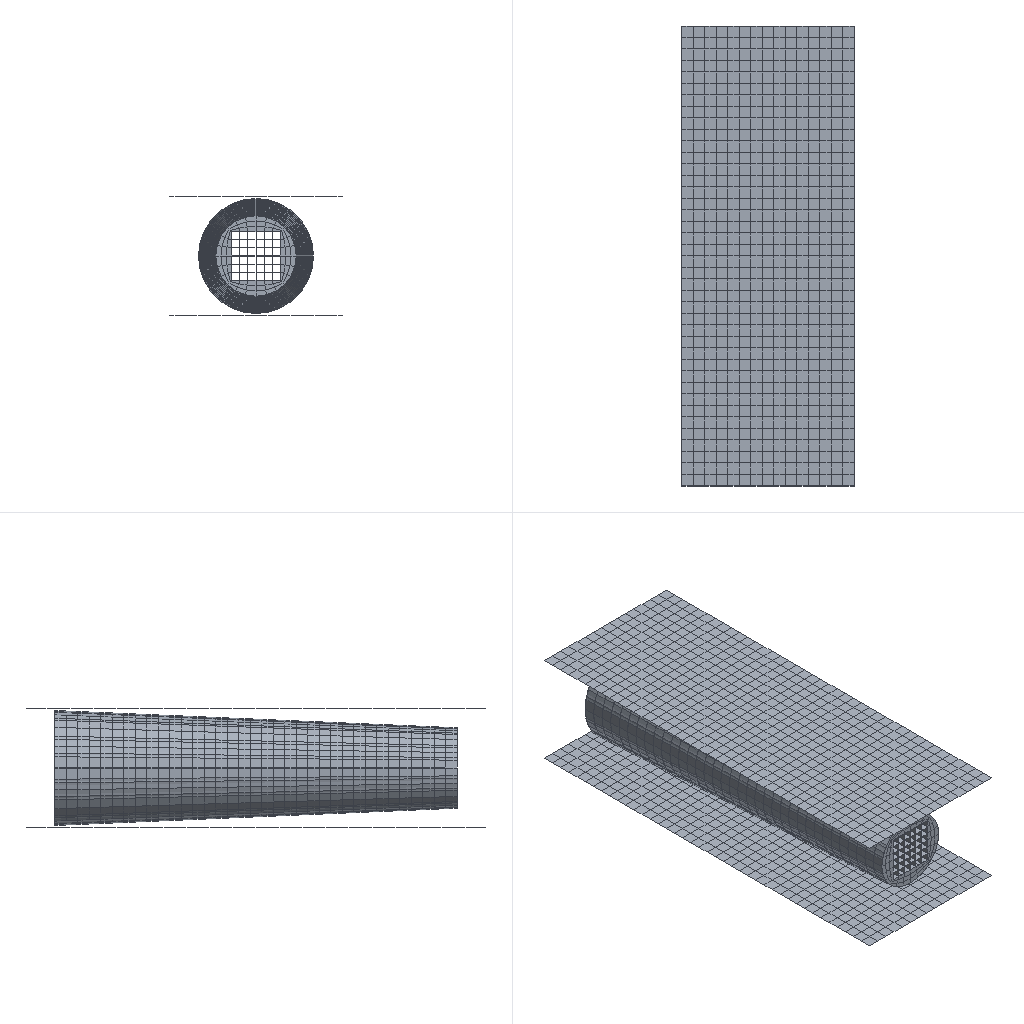Simulation study | abaqus
Set-up summary:
category,name,step,type,value,unit,region
solver,abaqus
solver,version,,,Abaqus/Explicit 2020
units,not stated in the deck,,not stated
analysis,deck,,transient,transient
load_step,Step-1,Step-1,transient
load_step,requested,,,1
mesh,nodes,,,8118
mesh,elements,,,7501
element_type,S4R,,shell,4980
element_type,MASS,,point,1
element_type,C3D8R,,solid,2520
load,load commands in deck,,count,1
bc,support commands in deck,,count,1
material,LV,,in results
material,PU,,in results
material,RIG,,in results
check,setup vs results,,match,"per instance, exact: element labels, types and connectivity; labels of the nodes the elements use; coordinates of those nodes at SINGLE_PRECISION in 4 of 6 instance(s)"
Abaqus input file, long lists of numbers shortened:
*Heading
** Job name: Job-1 Model name: Model-1
** Generated by: Abaqus/CAE 2020
*Preprint, echo=NO, model=NO, history=NO, contact=NO
**
** PARTS
**
*Part, name=ZFX
*Node
      1,         -14.,         -14.,         350.
      2,         -14.,         -14.,           0.
** (1618 more lines like these left out)
*Element, type=S4R
 1,   1,  91, 158,   4
 2,  91,  92, 157, 158
** (2098 more lines like these left out)
*Nset, nset=Set-1
    1,    2,    5,    6,    7,    8,    9,   10,   11,   12,   17,   18,   29,   30,   31,   32
   33,   34,   35,   36,   37,   38,   39,   40,   41,   42,   43,   44,   45,   46,   49,   50
** (75 more lines like these left out)
*Elset, elset=Set-1
   36,   37,   38,   39,   40,   41,   42,   43,   44,   45,   46,   47,   48,   49,   50,   51
   52,   53,   54,   55,   56,   57,   58,   59,   60,   61,   62,   63,   64,   65,   66,   67
** (71 more lines like these left out)
*Nset, nset=Set-2, generate
    1,  1620,     1
*Elset, elset=Set-2, generate
    1,  2100,     1
** Section: zfx
*Shell Section, elset=Set-2, material=LV
0.5, 5
*End Part
**
*Part, name=chongjimian
*Node
      1,        -200.,         -75.,           0.
      2,        -190.,         -75.,           0.
** (654 more lines like these left out)
*Element, type=S4R
  1,   1,   2,  43,  42
  2,   2,   3,  44,  43
** (598 more lines like these left out)
*Node
    657,           0.,           0.,           0.
*Nset, nset=chongjimian-RefPt_, internal
657,
*Nset, nset=Set-1
 657,
*Nset, nset=Set-4, generate
   1,  656,    1
*Elset, elset=Set-4, generate
   1,  600,    1
** Section: rig
*Shell Section, elset=Set-4, material=rig
1., 5
*Element, type=MASS, elset=Set-1_Inertia-1_
601, 657
*Mass, elset=Set-1_Inertia-1_
0.5,
*End Part
**
*Part, name=dimian
*Node
      1,        -200.,         -75.,           0.
      2,        -190.,         -75.,           0.
** (654 more lines like these left out)
*Element, type=S4R
  1,   1,   2,  43,  42
  2,   2,   3,  44,  43
** (598 more lines like these left out)
*Node
    657,           0.,           0.,           0.
*Nset, nset=dimian-RefPt_, internal
657,
*Nset, nset=Set-2, generate
   1,  656,    1
*Elset, elset=Set-2, generate
   1,  600,    1
** Section: rig
*Shell Section, elset=Set-2, material=rig
1., 5
*End Part
**
*Part, name=dpm2
*Node
      1,         -21.,           0.,         -21.
      2,          21.,           0.,         -21.
** (3454 more lines like these left out)
*Element, type=C3D8R
  1,  180,  895, 2097,  759,    1,   23,  419,  100
  2,  895,  896, 2098, 2097,   23,   24,  420,  419
** (2518 more lines like these left out)
*Nset, nset=Set-1, generate
    1,  3456,     1
*Elset, elset=Set-1, generate
    1,  2520,     1
** Section: PU
*Solid Section, elset=Set-1, material=PU
,
*End Part
**
*Part, name=fangguan
*Node
      1,         -21.,         -21.,         350.
      2,         -21.,          21.,         350.
** (574 more lines like these left out)
*Element, type=S4R
  1,   1,   9, 169,  82
  2,   9,  10, 170, 169
** (558 more lines like these left out)
*Nset, nset=Set-1, generate
   1,  576,    1
*Elset, elset=Set-1, generate
   1,  560,    1
** Section: fangguan
*Shell Section, elset=Set-1, material=LV, offset=SPOS
0.5, 5
*End Part
**
*Part, name=waike
*Node
      1,  -34.327,           0.,   6.828
      2,  -32.336,           0.,   13.394
** (1150 more lines like these left out)
*Element, type=S4R
   1,   32,    1,   33,   64
   2,    1,    2,   34,   33
** (1118 more lines like these left out)
*Nset, nset=Set-1, generate
    1,  1152,     1
*Elset, elset=Set-1, generate
    1,  1120,     1
** Section: waike
*Shell Section, elset=Set-1, material=LV, offset=SNEG
2., 5
*End Part
**
**
** ASSEMBLY
**
*Assembly, name=Assembly
**
*Instance, name=waike, part=waike
*End Instance
**
*Instance, name=chongjimian-1, part=chongjimian
          0.,         175.,          52.
          0.,         175.,          52.,           0.,         175., 53., 90.
*End Instance
**
*Instance, name=dimian-1, part=dimian
          0.,         175.,         -52.
          0.,         175.,         -52.,           0.,         175., -51., 90.
*End Instance
**
*Instance, name=ZFX-1, part=ZFX
          0.,           0.,           0.
          0.,           0.,           0., -1.,           0.,           0., 90.
*End Instance
**
*Instance, name=dpm2-1, part=dpm2
*End Instance
**
*Instance, name=fangguan-1, part=fangguan
          0.,           0.,           0.
          0.,           0.,           0., -1.,           0.,           0., 90.
*End Instance
**
*Nset, nset=Set-1, instance=chongjimian-1
 657,
*Nset, nset=Set-6, instance=dimian-1
 657,
*Nset, nset=b_Set-2, instance=dimian-1, generate
   1,  656,    1
*Elset, elset=b_Set-2, instance=dimian-1, generate
   1,  600,    1
*Nset, nset=b_Set-4, instance=chongjimian-1, generate
   1,  656,    1
*Elset, elset=b_Set-4, instance=chongjimian-1, generate
   1,  600,    1
*Nset, nset=_PickedSet24, internal, instance=dimian-1
 657,
*Nset, nset=_PickedSet26, internal, instance=chongjimian-1
 657,
** Constraint: Constraint-1
*Rigid Body, ref node=_PickedSet24, elset=b_Set-2
** Constraint: Constraint-2
*Rigid Body, ref node=_PickedSet26, elset=b_Set-4
*End Assembly
**
** MATERIALS
**
*Material, name=LV
*Density
 2.72e-09,
*Elastic
69000., 0.3
*Plastic
 80.,    0.
115., 0.024
139., 0.049
150., 0.074
158., 0.099
167., 0.124
171., 0.149
173., 0.174
*Material, name=PU
*Density
 4e-10,
*Hyperfoam, n=2, poisson=0., testdata
*Uniaxial Test Data
 -0.0217, -0.05,    0.
 -0.0317,  -0.1,    0.
 -0.0367, -0.15,    0.
 -0.0402,  -0.2,    0.
 -0.0433, -0.25,    0.
 -0.0467,  -0.3,    0.
 -0.0504, -0.35,    0.
 -0.0542,  -0.4,    0.
 -0.0604, -0.45,    0.
 -0.0668,  -0.5,    0.
*Material, name=rig
*Density
 7.8e-09,
*Elastic
210000., 0.3
**
** INTERACTION PROPERTIES
**
*Surface Interaction, name=IntProp-1
*Friction
 0.2,
*Surface Behavior, pressure-overclosure=HARD
**
** PREDEFINED FIELDS
**
** Name: Predefined Field-1   Type: Velocity
*Initial Conditions, type=VELOCITY
Set-1, 1, 0.
Set-1, 2, 0.
Set-1, 3, -7500.
**
** INTERACTIONS
**
** Interaction: Int-1
*Contact, op=NEW
*Contact Inclusions, ALL EXTERIOR
*Contact Property Assignment
 ,  , IntProp-1
** ----------------------------------------------------------------
**
** STEP: Step-1
**
*Step, name=Step-1, nlgeom=YES
*Dynamic, Explicit
, 0.01
*Bulk Viscosity
0.06, 1.2
** Mass Scaling: Semi-Automatic
**               Whole Model
*Fixed Mass Scaling, factor=500.
**
** BOUNDARY CONDITIONS
**
** Name: BC-1 Type: 对称/反对称/完全固定
*Boundary
Set-6, ENCASTRE
**
** OUTPUT REQUESTS
**
*Restart, write, number interval=1, time marks=NO
**
** FIELD OUTPUT: F-Output-1
**
*Output, field, number interval=50
*Node Output
A, CF, RF, RM, RT, U, V
*Element Output, directions=YES
E, EVF, LE, MISES, MISESMAX, PE, PEEQ, PEEQMAX, PEEQT, PEEQVAVG, PEMAG, PEVAVG, S, SF, SVAVG
*Contact Output
CDISP, CSTRESS
**
** HISTORY OUTPUT: H-Output-1
**
*Output, history, time interval=5e-06
*Node Output, nset=Set-6
RF3,
*End Step
Results summary:
result,step,Step-1,completed,increments=3828 time=0.01/0.01
result,analysis,,,transient
result,last_loadstep,,,1
result,primary field,,,"U, UR"
result,reaction total,,FX,17810.771,model units
result,reaction total,,FY,-3880.226,model units
result,reaction total,,FZ,689803.062,model units